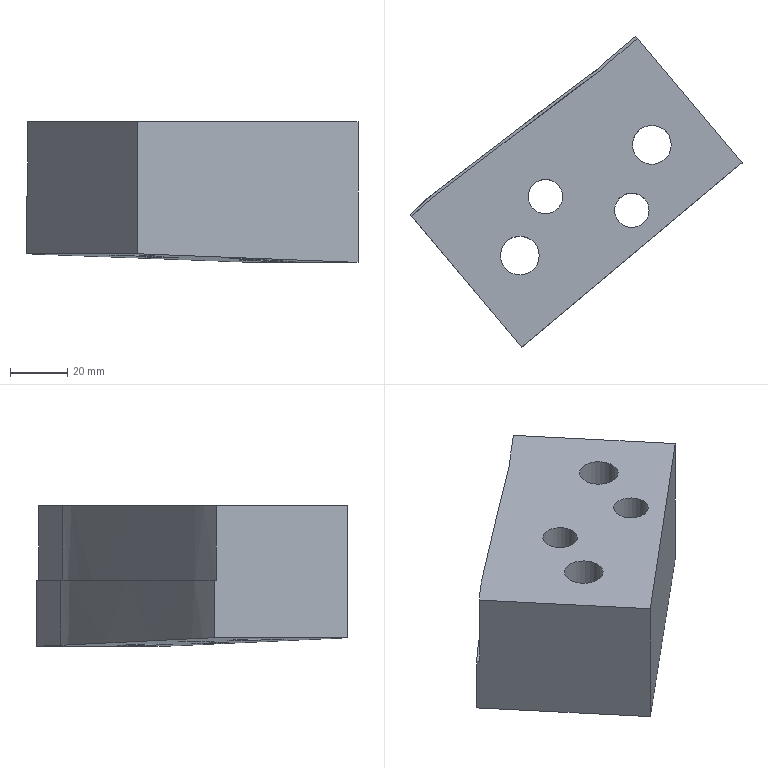Part | NX | features solid 2 | 1 solid | 22 faces | box 115.597 x 108.38 x 49 mm | volume 247805 mm3 | plane 12 | cylinder 8 | spline 2 | commonest cylinder face diameters 12 x2 13 x2 13.5 x2 19.5 x2
STEP:
#1=CARTESIAN_POINT('',(398.511,3.234,40.));
#2=VERTEX_POINT('',#1);
#3=CARTESIAN_POINT('',(408.585,11.687,40.));
#4=VERTEX_POINT('',#3);
#5=CARTESIAN_POINT('',(-63.471,-384.415,40.));
#6=DIRECTION('',(0.766,0.6428,0.));
#7=VECTOR('',#6,1000.);
#8=LINE('',#5,#7);
#9=EDGE_CURVE('',#2,#4,#8,.T.);
#10=ORIENTED_EDGE('',*,*,#9,.F.);
#11=CARTESIAN_POINT('',(329.994,-50.225,40.));
#12=VERTEX_POINT('',#11);
#13=CARTESIAN_POINT('',(329.994,-50.225,40.));
#14=CARTESIAN_POINT('',(331.334,-49.01,40.));
#15=CARTESIAN_POINT('',(333.889,-46.435,40.));
#16=CARTESIAN_POINT('',(338.043,-42.95,40.));
#17=CARTESIAN_POINT('',(342.497,-39.816,40.));
#18=CARTESIAN_POINT('',(346.834,-36.54,40.));
#19=CARTESIAN_POINT('',(351.16,-33.247,40.));
#20=CARTESIAN_POINT('',(356.896,-28.814,40.));
#21=CARTESIAN_POINT('',(364.051,-23.254,40.));
#22=CARTESIAN_POINT('',(372.649,-16.597,40.));
#23=CARTESIAN_POINT('',(379.858,-11.107,40.));
#24=CARTESIAN_POINT('',(385.676,-6.784,40.));
#25=CARTESIAN_POINT('',(390.076,-3.582,40.));
#26=CARTESIAN_POINT('',(394.468,-0.4036,40.));
#27=CARTESIAN_POINT('',(397.371,1.834,40.));
#28=CARTESIAN_POINT('',(398.511,3.234,40.));
#29=B_SPLINE_CURVE_WITH_KNOTS('',3,(#13,#14,#15,#16,#17,#18,#19,#20,#21,#22,#23,#24,#25,#26,#27,#28),.UNSPECIFIED.,.F.,.F.,(4,1,1,1,1,1,1,1,1,1,1,1,1,4),(0.001774,0.007197,0.01262,0.01804,0.02346,0.02889,0.03431,0.04515,0.056,0.06685,0.07227,0.07769,0.08311,0.08854),.UNSPECIFIED.);
#30=EDGE_CURVE('',#12,#2,#29,.T.);
#31=ORIENTED_EDGE('',*,*,#30,.F.);
#32=CARTESIAN_POINT('',(368.343,-95.927,40.));
#33=VERTEX_POINT('',#32);
#34=CARTESIAN_POINT('',(-20.026,366.913,40.));
#35=DIRECTION('',(-0.6428,0.766,0.));
#36=VECTOR('',#35,1000.);
#37=LINE('',#34,#36);
#38=EDGE_CURVE('',#33,#12,#37,.T.);
#39=ORIENTED_EDGE('',*,*,#38,.F.);
#40=CARTESIAN_POINT('',(444.947,-31.649,40.));
#41=VERTEX_POINT('',#40);
#42=CARTESIAN_POINT('',(628.198,122.117,40.));
#43=DIRECTION('',(0.766,0.6428,0.));
#44=VECTOR('',#43,1000.);
#45=LINE('',#42,#44);
#46=EDGE_CURVE('',#33,#41,#45,.T.);
#47=ORIENTED_EDGE('',*,*,#46,.T.);
#48=CARTESIAN_POINT('',(56.578,431.192,40.));
#49=DIRECTION('',(-0.6428,0.766,0.));
#50=VECTOR('',#49,1000.);
#51=LINE('',#48,#50);
#52=EDGE_CURVE('',#41,#4,#51,.T.);
#53=ORIENTED_EDGE('',*,*,#52,.T.);
#54=EDGE_LOOP('',(#10,#31,#39,#47,#53));
#55=FACE_BOUND('',#54,.T.);
#56=CARTESIAN_POINT('',(374.344,-63.92,40.));
#57=VERTEX_POINT('',#56);
#58=CARTESIAN_POINT('',(367.594,-63.92,40.));
#59=DIRECTION('',(0.,0.,1.));
#60=DIRECTION('',(1.,0.,0.));
#61=AXIS2_PLACEMENT_3D('',#58,#59,#60);
#62=CIRCLE('',#61,6.75);
#63=EDGE_CURVE('',#57,#57,#62,.T.);
#64=ORIENTED_EDGE('',*,*,#63,.F.);
#65=EDGE_LOOP('',(#64));
#66=FACE_BOUND('',#65,.T.);
#67=CARTESIAN_POINT('',(420.307,-25.353,40.));
#68=VERTEX_POINT('',#67);
#69=CARTESIAN_POINT('',(413.557,-25.353,40.));
#70=DIRECTION('',(0.,0.,1.));
#71=DIRECTION('',(1.,0.,0.));
#72=AXIS2_PLACEMENT_3D('',#69,#70,#71);
#73=CIRCLE('',#72,6.75);
#74=EDGE_CURVE('',#68,#68,#73,.T.);
#75=ORIENTED_EDGE('',*,*,#74,.F.);
#76=EDGE_LOOP('',(#75));
#77=FACE_BOUND('',#76,.T.);
#78=CARTESIAN_POINT('',(412.592,-48.168,40.));
#79=VERTEX_POINT('',#78);
#80=CARTESIAN_POINT('',(406.592,-48.168,40.));
#81=DIRECTION('',(0.,0.,1.));
#82=DIRECTION('',(1.,0.,0.));
#83=AXIS2_PLACEMENT_3D('',#80,#81,#82);
#84=CIRCLE('',#83,6.);
#85=EDGE_CURVE('',#79,#79,#84,.T.);
#86=ORIENTED_EDGE('',*,*,#85,.F.);
#87=EDGE_LOOP('',(#86));
#88=FACE_BOUND('',#87,.T.);
#89=CARTESIAN_POINT('',(382.487,-43.404,40.));
#90=VERTEX_POINT('',#89);
#91=CARTESIAN_POINT('',(376.487,-43.404,40.));
#92=DIRECTION('',(0.,0.,1.));
#93=DIRECTION('',(1.,0.,0.));
#94=AXIS2_PLACEMENT_3D('',#91,#92,#93);
#95=CIRCLE('',#94,6.);
#96=EDGE_CURVE('',#90,#90,#95,.T.);
#97=ORIENTED_EDGE('',*,*,#96,.F.);
#98=EDGE_LOOP('',(#97));
#99=FACE_BOUND('',#98,.T.);
#100=CARTESIAN_POINT('',(-415.478,35.09,40.));
#101=DIRECTION('',(0.,0.,1.));
#102=DIRECTION('',(1.,0.,0.));
#103=AXIS2_PLACEMENT_3D('',#100,#101,#102);
#104=PLANE('',#103);
#105=ADVANCED_FACE('',(#55,#66,#77,#88,#99),#104,.T.);
#106=CARTESIAN_POINT('',(397.794,3.938,14.));
#107=VERTEX_POINT('',#106);
#108=CARTESIAN_POINT('',(329.35,-49.458,14.));
#109=VERTEX_POINT('',#108);
#110=CARTESIAN_POINT('',(-190.231,-121.49,14.));
#111=CARTESIAN_POINT('',(-188.654,-121.152,14.));
#112=CARTESIAN_POINT('',(-185.47,-120.627,14.));
#113=CARTESIAN_POINT('',(-180.656,-120.141,14.));
#114=CARTESIAN_POINT('',(-175.882,-119.326,14.));
#115=CARTESIAN_POINT('',(-169.679,-117.528,14.));
#116=CARTESIAN_POINT('',(-162.185,-114.539,14.));
#117=CARTESIAN_POINT('',(-153.086,-111.254,14.));
#118=CARTESIAN_POINT('',(-144.031,-107.845,14.));
#119=CARTESIAN_POINT('',(-136.465,-105.061,14.));
#120=CARTESIAN_POINT('',(-130.418,-102.814,14.));
#121=CARTESIAN_POINT('',(-125.812,-101.329,14.));
#122=CARTESIAN_POINT('',(-121.306,-99.566,14.));
#123=CARTESIAN_POINT('',(-116.876,-97.626,14.));
#124=CARTESIAN_POINT('',(-112.335,-95.923,14.));
#125=CARTESIAN_POINT('',(-107.564,-95.05,14.));
#126=CARTESIAN_POINT('',(-102.756,-94.525,14.));
#127=CARTESIAN_POINT('',(-96.349,-93.771,14.));
#128=CARTESIAN_POINT('',(-89.902,-93.468,14.));
#129=CARTESIAN_POINT('',(-83.452,-93.448,14.));
#130=CARTESIAN_POINT('',(-77.002,-93.469,14.));
#131=CARTESIAN_POINT('',(-68.939,-93.411,14.));
#132=CARTESIAN_POINT('',(-56.04,-93.3,14.));
#133=CARTESIAN_POINT('',(-33.465,-93.184,14.));
#134=CARTESIAN_POINT('',(-7.666,-93.074,14.));
#135=CARTESIAN_POINT('',(14.907,-92.653,14.));
#136=CARTESIAN_POINT('',(27.794,-92.068,14.));
#137=CARTESIAN_POINT('',(40.668,-91.245,14.));
#138=CARTESIAN_POINT('',(51.917,-90.291,14.));
#139=CARTESIAN_POINT('',(61.528,-89.174,14.));
#140=CARTESIAN_POINT('',(67.939,-88.466,14.));
#141=CARTESIAN_POINT('',(79.125,-86.95,14.));
#142=CARTESIAN_POINT('',(95.161,-85.253,14.));
#143=CARTESIAN_POINT('',(114.404,-83.21,14.));
#144=CARTESIAN_POINT('',(133.568,-80.524,14.));
#145=CARTESIAN_POINT('',(152.734,-77.861,14.));
#146=CARTESIAN_POINT('',(171.916,-75.326,14.));
#147=CARTESIAN_POINT('',(191.055,-72.413,14.));
#148=CARTESIAN_POINT('',(207.17,-71.468,14.));
#149=CARTESIAN_POINT('',(219.951,-69.697,14.));
#150=CARTESIAN_POINT('',(232.724,-67.899,14.));
#151=CARTESIAN_POINT('',(248.708,-65.766,14.));
#152=CARTESIAN_POINT('',(267.87,-63.074,14.));
#153=CARTESIAN_POINT('',(287.038,-60.44,14.));
#154=CARTESIAN_POINT('',(301.448,-58.682,14.));
#155=CARTESIAN_POINT('',(310.976,-56.987,14.));
#156=CARTESIAN_POINT('',(314.916,-56.135,14.));
#157=CARTESIAN_POINT('',(318.052,-55.382,14.));
#158=CARTESIAN_POINT('',(320.39,-54.76,14.));
#159=CARTESIAN_POINT('',(322.686,-53.981,14.));
#160=CARTESIAN_POINT('',(325.595,-52.578,14.));
#161=CARTESIAN_POINT('',(328.769,-50.098,14.));
#162=CARTESIAN_POINT('',(332.247,-46.69,14.));
#163=CARTESIAN_POINT('',(335.795,-43.406,14.));
#164=CARTESIAN_POINT('',(343.661,-37.758,14.));
#165=CARTESIAN_POINT('',(355.164,-28.914,14.));
#166=CARTESIAN_POINT('',(370.422,-17.018,14.));
#167=CARTESIAN_POINT('',(383.264,-7.249,14.));
#168=CARTESIAN_POINT('',(392.416,-0.6713,14.));
#169=CARTESIAN_POINT('',(396.953,2.733,14.));
#170=CARTESIAN_POINT('',(398.886,5.372,14.));
#171=CARTESIAN_POINT('',(399.725,7.654,14.));
#172=CARTESIAN_POINT('',(399.76,10.078,14.));
#173=CARTESIAN_POINT('',(399.483,13.317,14.));
#174=CARTESIAN_POINT('',(399.712,17.34,14.));
#175=CARTESIAN_POINT('',(399.612,22.179,14.));
#176=CARTESIAN_POINT('',(399.633,31.854,14.));
#177=CARTESIAN_POINT('',(399.593,46.366,14.));
#178=CARTESIAN_POINT('',(399.637,62.491,14.));
#179=CARTESIAN_POINT('',(399.588,73.779,14.));
#180=CARTESIAN_POINT('',(399.652,79.422,14.));
#181=CARTESIAN_POINT('',(399.59,82.647,14.));
#182=CARTESIAN_POINT('',(399.564,85.065,14.));
#183=CARTESIAN_POINT('',(399.725,87.486,14.));
#184=CARTESIAN_POINT('',(399.756,89.902,14.));
#185=CARTESIAN_POINT('',(399.247,92.301,14.));
#186=CARTESIAN_POINT('',(397.362,95.008,14.));
#187=CARTESIAN_POINT('',(393.635,96.774,14.));
#188=CARTESIAN_POINT('',(389.279,98.826,14.));
#189=CARTESIAN_POINT('',(384.732,100.498,14.));
#190=CARTESIAN_POINT('',(378.765,102.95,14.));
#191=CARTESIAN_POINT('',(362.589,110.229,14.));
#192=CARTESIAN_POINT('',(344.928,118.135,14.));
#193=CARTESIAN_POINT('',(327.281,126.072,14.));
#194=CARTESIAN_POINT('',(319.932,129.381,14.));
#195=CARTESIAN_POINT('',(314.075,132.102,14.));
#196=CARTESIAN_POINT('',(309.387,133.376,14.));
#197=CARTESIAN_POINT('',(304.547,133.785,14.));
#198=CARTESIAN_POINT('',(299.716,133.401,14.));
#199=CARTESIAN_POINT('',(294.929,132.704,14.));
#200=CARTESIAN_POINT('',(288.543,131.8,14.));
#201=CARTESIAN_POINT('',(277.364,130.241,14.));
#202=CARTESIAN_POINT('',(242.2,125.552,14.));
#203=CARTESIAN_POINT('',(184.637,118.048,14.));
#204=CARTESIAN_POINT('',(120.701,109.541,14.));
#205=CARTESIAN_POINT('',(69.531,102.902,14.));
#206=CARTESIAN_POINT('',(40.777,98.94,14.));
#207=CARTESIAN_POINT('',(21.566,96.615,14.));
#208=CARTESIAN_POINT('',(8.743,95.212,14.));
#209=CARTESIAN_POINT('',(-7.301,93.575,14.));
#210=CARTESIAN_POINT('',(-26.625,92.505,14.));
#211=CARTESIAN_POINT('',(-45.971,92.017,14.));
#212=CARTESIAN_POINT('',(-62.09,91.675,14.));
#213=CARTESIAN_POINT('',(-74.987,91.256,14.));
#214=CARTESIAN_POINT('',(-84.664,91.165,14.));
#215=CARTESIAN_POINT('',(-94.319,91.781,14.));
#216=CARTESIAN_POINT('',(-103.929,92.966,14.));
#217=CARTESIAN_POINT('',(-113.495,94.403,14.));
#218=CARTESIAN_POINT('',(-119.856,95.492,14.));
#219=CARTESIAN_POINT('',(-122.997,96.222,14.));
#220=B_SPLINE_CURVE_WITH_KNOTS('',3,(#110,#111,#112,#113,#114,#115,#116,#117,#118,#119,#120,#121,#122,#123,#124,#125,#126,#127,#128,#129,#130,#131,#132,#133,#134,#135,#136,#137,#138,#139,#140,#141,#142,#143,#144,#145,#146,#147,#148,#149,#150,#151,#152,#153,#154,#155,#156,#157,#158,#159,#160,#161,#162,#163,#164,#165,#166,#167,#168,#169,#170,#171,#172,#173,#174,#175,#176,#177,#178,#179,#180,#181,#182,#183,#184,#185,#186,#187,#188,#189,#190,#191,#192,#193,#194,#195,#196,#197,#198,#199,#200,#201,#202,#203,#204,#205,#206,#207,#208,#209,#210,#211,#212,#213,#214,#215,#216,#217,#218,#219),.UNSPECIFIED.,.F.,.F.,(4,1,1,1,1,1,1,1,1,1,1,1,1,1,1,1,1,1,1,1,1,1,1,1,1,1,1,1,1,1,1,1,1,1,1,1,1,1,1,1,1,1,1,1,1,1,1,1,1,1,1,1,1,1,1,1,1,1,1,1,1,1,1,1,1,1,1,1,1,1,1,1,1,1,1,1,1,1,1,1,1,1,1,1,1,1,1,1,1,1,1,1,1,1,1,1,1,1,1,1,1,1,1,1,1,1,1,4),(0.4704,0.4724,0.4745,0.4766,0.4786,0.4828,0.4869,0.491,0.4952,0.4972,0.4993,0.5014,0.5035,0.5055,0.5076,0.5097,0.5117,0.5159,0.5179,0.52,0.5241,0.5283,0.5366,0.5531,0.5614,0.5655,0.5697,0.5779,0.58,0.5821,0.5862,0.5945,0.6028,0.611,0.6193,0.6276,0.6359,0.6441,0.6483,0.6524,0.6607,0.669,0.6772,0.6855,0.6876,0.6897,0.6907,0.6917,0.6928,0.6938,0.6959,0.6979,0.7,0.7021,0.7103,0.7186,0.7269,0.731,0.7331,0.7341,0.7352,0.7362,0.7372,0.7393,0.7414,0.7435,0.7517,0.76,0.7641,0.7662,0.7672,0.7683,0.7693,0.7703,0.7714,0.7724,0.7745,0.7766,0.7786,0.7807,0.7848,0.8014,0.8055,0.8097,0.8117,0.8138,0.8159,0.8179,0.82,0.8221,0.8262,0.8345,0.8676,0.9007,0.9172,0.9338,0.9379,0.9421,0.9503,0.9586,0.9669,0.9752,0.9793,0.9834,0.9876,0.9917,0.9959,1.),.UNSPECIFIED.);
#221=EDGE_CURVE('',#107,#109,#220,.F.);
#222=ORIENTED_EDGE('',*,*,#221,.F.);
#223=CARTESIAN_POINT('',(397.794,3.938,-8.603));
#224=VERTEX_POINT('',#223);
#225=CARTESIAN_POINT('',(397.794,3.938,15.353));
#226=DIRECTION('',(0.,0.,-1.));
#227=VECTOR('',#226,1000.);
#228=LINE('',#225,#227);
#229=EDGE_CURVE('',#107,#224,#228,.T.);
#230=ORIENTED_EDGE('',*,*,#229,.T.);
#231=CARTESIAN_POINT('',(329.35,-49.458,-6.));
#232=VERTEX_POINT('',#231);
#233=CARTESIAN_POINT('',(397.794,3.938,-8.603));
#234=CARTESIAN_POINT('',(396.669,2.533,-8.55));
#235=CARTESIAN_POINT('',(393.753,0.322,-8.44));
#236=CARTESIAN_POINT('',(389.372,-2.859,-8.278));
#237=CARTESIAN_POINT('',(384.978,-6.055,-8.115));
#238=CARTESIAN_POINT('',(379.17,-10.374,-7.899));
#239=CARTESIAN_POINT('',(371.973,-15.855,-7.627));
#240=CARTESIAN_POINT('',(363.39,-22.501,-7.302));
#241=CARTESIAN_POINT('',(356.247,-28.052,-7.031));
#242=CARTESIAN_POINT('',(350.521,-32.477,-6.814));
#243=CARTESIAN_POINT('',(346.202,-35.764,-6.651));
#244=CARTESIAN_POINT('',(341.87,-39.036,-6.489));
#245=CARTESIAN_POINT('',(337.427,-42.164,-6.326));
#246=CARTESIAN_POINT('',(333.263,-45.65,-6.163));
#247=CARTESIAN_POINT('',(330.694,-48.239,-6.054));
#248=CARTESIAN_POINT('',(329.35,-49.458,-6.));
#249=B_SPLINE_CURVE_WITH_KNOTS('',3,(#233,#234,#235,#236,#237,#238,#239,#240,#241,#242,#243,#244,#245,#246,#247,#248),.UNSPECIFIED.,.F.,.F.,(4,1,1,1,1,1,1,1,1,1,1,1,1,4),(0.01887,0.02429,0.02971,0.03513,0.04055,0.05139,0.06223,0.07307,0.07849,0.08391,0.08933,0.09475,0.1002,0.1056),.UNSPECIFIED.);
#250=EDGE_CURVE('',#224,#232,#249,.T.);
#251=ORIENTED_EDGE('',*,*,#250,.T.);
#252=CARTESIAN_POINT('',(329.35,-49.458,4.));
#253=DIRECTION('',(0.,0.,-1.));
#254=VECTOR('',#253,1000.);
#255=LINE('',#252,#254);
#256=EDGE_CURVE('',#109,#232,#255,.T.);
#257=ORIENTED_EDGE('',*,*,#256,.F.);
#258=EDGE_LOOP('',(#222,#230,#251,#257));
#259=FACE_BOUND('',#258,.T.);
#260=CARTESIAN_POINT('',(329.35,-49.458,14.));
#261=CARTESIAN_POINT('',(329.35,-49.458,-8.738));
#262=CARTESIAN_POINT('',(330.694,-48.239,14.));
#263=CARTESIAN_POINT('',(330.694,-48.239,-8.738));
#264=CARTESIAN_POINT('',(333.261,-45.653,14.));
#265=CARTESIAN_POINT('',(333.261,-45.653,-8.738));
#266=CARTESIAN_POINT('',(337.411,-42.175,14.));
#267=CARTESIAN_POINT('',(337.411,-42.175,-8.738));
#268=CARTESIAN_POINT('',(341.859,-39.044,14.));
#269=CARTESIAN_POINT('',(341.859,-39.044,-8.738));
#270=CARTESIAN_POINT('',(346.191,-35.773,14.));
#271=CARTESIAN_POINT('',(346.191,-35.773,-8.738));
#272=CARTESIAN_POINT('',(350.51,-32.485,14.));
#273=CARTESIAN_POINT('',(350.51,-32.485,-8.738));
#274=CARTESIAN_POINT('',(356.237,-28.06,14.));
#275=CARTESIAN_POINT('',(356.237,-28.06,-8.738));
#276=CARTESIAN_POINT('',(363.38,-22.509,14.));
#277=CARTESIAN_POINT('',(363.38,-22.509,-8.738));
#278=CARTESIAN_POINT('',(371.966,-15.861,14.));
#279=CARTESIAN_POINT('',(371.966,-15.861,-8.738));
#280=CARTESIAN_POINT('',(379.167,-10.376,14.));
#281=CARTESIAN_POINT('',(379.167,-10.376,-8.738));
#282=CARTESIAN_POINT('',(384.974,-6.058,14.));
#283=CARTESIAN_POINT('',(384.974,-6.058,-8.738));
#284=CARTESIAN_POINT('',(389.359,-2.869,14.));
#285=CARTESIAN_POINT('',(389.359,-2.869,-8.738));
#286=CARTESIAN_POINT('',(393.75,0.3223,14.));
#287=CARTESIAN_POINT('',(393.75,0.3223,-8.738));
#288=CARTESIAN_POINT('',(396.658,2.52,14.));
#289=CARTESIAN_POINT('',(396.658,2.52,-8.738));
#290=CARTESIAN_POINT('',(397.794,3.938,14.));
#291=CARTESIAN_POINT('',(397.794,3.938,-8.738));
#292=B_SPLINE_SURFACE_WITH_KNOTS('',3,1,((#260,#261),(#262,#263),(#264,#265),(#266,#267),(#268,#269),(#270,#271),(#272,#273),(#274,#275),(#276,#277),(#278,#279),(#280,#281),(#282,#283),(#284,#285),(#286,#287),(#288,#289),(#290,#291)),.SURF_OF_LINEAR_EXTRUSION.,.F.,.F.,.F.,(4,1,1,1,1,1,1,1,1,1,1,1,1,4),(2,2),(0.6962,0.6986,0.7009,0.7032,0.7055,0.7078,0.7102,0.7148,0.7194,0.7241,0.7264,0.7287,0.7311,0.7334),(0.,1.),.UNSPECIFIED.);
#293=ADVANCED_FACE('',(#259),#292,.T.);
#294=CARTESIAN_POINT('',(408.585,11.687,14.));
#295=VERTEX_POINT('',#294);
#296=CARTESIAN_POINT('',(407.942,12.453,14.));
#297=VERTEX_POINT('',#296);
#298=CARTESIAN_POINT('',(608.355,-226.39,14.));
#299=DIRECTION('',(-0.6428,0.766,0.));
#300=VECTOR('',#299,1000.);
#301=LINE('',#298,#300);
#302=EDGE_CURVE('',#295,#297,#301,.T.);
#303=ORIENTED_EDGE('',*,*,#302,.F.);
#304=CARTESIAN_POINT('',(408.585,11.687,2.));
#305=DIRECTION('',(0.,0.,-1.));
#306=VECTOR('',#305,1000.);
#307=LINE('',#304,#306);
#308=EDGE_CURVE('',#4,#295,#307,.T.);
#309=ORIENTED_EDGE('',*,*,#308,.F.);
#310=ORIENTED_EDGE('',*,*,#52,.F.);
#311=CARTESIAN_POINT('',(444.947,-31.649,-9.));
#312=VERTEX_POINT('',#311);
#313=CARTESIAN_POINT('',(444.947,-31.649,2.));
#314=DIRECTION('',(0.,0.,1.));
#315=VECTOR('',#314,1000.);
#316=LINE('',#313,#315);
#317=EDGE_CURVE('',#312,#41,#316,.T.);
#318=ORIENTED_EDGE('',*,*,#317,.F.);
#319=CARTESIAN_POINT('',(407.942,12.453,-9.));
#320=VERTEX_POINT('',#319);
#321=CARTESIAN_POINT('',(160.485,307.36,-9.));
#322=DIRECTION('',(0.6428,-0.766,0.));
#323=VECTOR('',#322,1000.);
#324=LINE('',#321,#323);
#325=EDGE_CURVE('',#320,#312,#324,.T.);
#326=ORIENTED_EDGE('',*,*,#325,.F.);
#327=CARTESIAN_POINT('',(407.942,12.453,100.));
#328=DIRECTION('',(0.,0.,1.));
#329=VECTOR('',#328,1000.);
#330=LINE('',#327,#329);
#331=EDGE_CURVE('',#297,#320,#330,.F.);
#332=ORIENTED_EDGE('',*,*,#331,.F.);
#333=EDGE_LOOP('',(#303,#309,#310,#318,#326,#332));
#334=FACE_BOUND('',#333,.T.);
#335=CARTESIAN_POINT('',(608.355,-226.39,2.));
#336=DIRECTION('',(0.766,0.6428,0.));
#337=DIRECTION('',(-0.6428,0.766,0.));
#338=AXIS2_PLACEMENT_3D('',#335,#336,#337);
#339=PLANE('',#338);
#340=ADVANCED_FACE('',(#334),#339,.T.);
#341=CARTESIAN_POINT('',(381.466,-39.226,-7.395));
#342=VERTEX_POINT('',#341);
#343=CARTESIAN_POINT('',(376.487,-43.404,-7.2));
#344=DIRECTION('',(-0.02297,-0.01927,-0.9996));
#345=DIRECTION('',(0.7657,0.6425,-0.02999));
#346=AXIS2_PLACEMENT_3D('',#343,#344,#345);
#347=ELLIPSE('',#346,6.503,6.5);
#348=EDGE_CURVE('',#342,#342,#347,.T.);
#349=ORIENTED_EDGE('',*,*,#348,.F.);
#350=EDGE_LOOP('',(#349));
#351=FACE_BOUND('',#350,.T.);
#352=CARTESIAN_POINT('',(411.571,-43.989,-7.995));
#353=VERTEX_POINT('',#352);
#354=CARTESIAN_POINT('',(406.592,-48.168,-7.8));
#355=DIRECTION('',(-0.02297,-0.01927,-0.9996));
#356=DIRECTION('',(0.7657,0.6425,-0.02999));
#357=AXIS2_PLACEMENT_3D('',#354,#355,#356);
#358=ELLIPSE('',#357,6.503,6.5);
#359=EDGE_CURVE('',#353,#353,#358,.T.);
#360=ORIENTED_EDGE('',*,*,#359,.F.);
#361=EDGE_LOOP('',(#360));
#362=FACE_BOUND('',#361,.T.);
#363=CARTESIAN_POINT('',(421.026,-19.086,-8.693));
#364=VERTEX_POINT('',#363);
#365=CARTESIAN_POINT('',(413.557,-25.353,-8.4));
#366=DIRECTION('',(-0.02297,-0.01927,-0.9996));
#367=DIRECTION('',(0.7657,0.6425,-0.02999));
#368=AXIS2_PLACEMENT_3D('',#365,#366,#367);
#369=ELLIPSE('',#368,9.754,9.75);
#370=EDGE_CURVE('',#364,#364,#369,.T.);
#371=ORIENTED_EDGE('',*,*,#370,.F.);
#372=EDGE_LOOP('',(#371));
#373=FACE_BOUND('',#372,.T.);
#374=CARTESIAN_POINT('',(375.063,-57.653,-6.893));
#375=VERTEX_POINT('',#374);
#376=CARTESIAN_POINT('',(367.594,-63.92,-6.6));
#377=DIRECTION('',(-0.02297,-0.01927,-0.9996));
#378=DIRECTION('',(0.7657,0.6425,-0.02999));
#379=AXIS2_PLACEMENT_3D('',#376,#377,#378);
#380=ELLIPSE('',#379,9.754,9.75);
#381=EDGE_CURVE('',#375,#375,#380,.T.);
#382=ORIENTED_EDGE('',*,*,#381,.F.);
#383=EDGE_LOOP('',(#382));
#384=FACE_BOUND('',#383,.T.);
#385=ORIENTED_EDGE('',*,*,#250,.F.);
#386=CARTESIAN_POINT('',(331.337,-51.826,-6.));
#387=DIRECTION('',(0.7657,0.6425,-0.02999));
#388=VECTOR('',#387,1000.);
#389=LINE('',#386,#388);
#390=EDGE_CURVE('',#224,#320,#389,.T.);
#391=ORIENTED_EDGE('',*,*,#390,.T.);
#392=ORIENTED_EDGE('',*,*,#325,.T.);
#393=CARTESIAN_POINT('',(368.343,-95.927,-6.));
#394=VERTEX_POINT('',#393);
#395=CARTESIAN_POINT('',(627.965,121.921,-16.167));
#396=DIRECTION('',(0.7657,0.6425,-0.02999));
#397=VECTOR('',#396,1000.);
#398=LINE('',#395,#397);
#399=EDGE_CURVE('',#394,#312,#398,.T.);
#400=ORIENTED_EDGE('',*,*,#399,.F.);
#401=CARTESIAN_POINT('',(83.881,243.081,-6.));
#402=DIRECTION('',(0.6428,-0.766,0.));
#403=VECTOR('',#402,1000.);
#404=LINE('',#401,#403);
#405=EDGE_CURVE('',#232,#394,#404,.T.);
#406=ORIENTED_EDGE('',*,*,#405,.F.);
#407=EDGE_LOOP('',(#385,#391,#392,#400,#406));
#408=FACE_BOUND('',#407,.T.);
#409=CARTESIAN_POINT('',(368.343,-95.927,-6.));
#410=DIRECTION('',(-0.02297,-0.01927,-0.9996));
#411=DIRECTION('',(-0.9997,0.,0.02298));
#412=AXIS2_PLACEMENT_3D('',#409,#410,#411);
#413=PLANE('',#412);
#414=ADVANCED_FACE('',(#351,#362,#373,#384,#408),#413,.T.);
#415=CARTESIAN_POINT('',(329.994,-50.225,14.));
#416=VERTEX_POINT('',#415);
#417=CARTESIAN_POINT('',(329.994,-50.225,57.));
#418=DIRECTION('',(0.,0.,1.));
#419=VECTOR('',#418,1000.);
#420=LINE('',#417,#419);
#421=EDGE_CURVE('',#12,#416,#420,.F.);
#422=ORIENTED_EDGE('',*,*,#421,.T.);
#423=CARTESIAN_POINT('',(354.158,-79.022,14.));
#424=DIRECTION('',(-0.6428,0.766,0.));
#425=VECTOR('',#424,1000.);
#426=LINE('',#423,#425);
#427=EDGE_CURVE('',#416,#109,#426,.T.);
#428=ORIENTED_EDGE('',*,*,#427,.T.);
#429=ORIENTED_EDGE('',*,*,#256,.T.);
#430=ORIENTED_EDGE('',*,*,#405,.T.);
#431=CARTESIAN_POINT('',(368.343,-95.927,23.));
#432=DIRECTION('',(0.,0.,1.));
#433=VECTOR('',#432,1000.);
#434=LINE('',#431,#433);
#435=EDGE_CURVE('',#394,#33,#434,.T.);
#436=ORIENTED_EDGE('',*,*,#435,.T.);
#437=ORIENTED_EDGE('',*,*,#38,.T.);
#438=EDGE_LOOP('',(#422,#428,#429,#430,#436,#437));
#439=FACE_BOUND('',#438,.T.);
#440=CARTESIAN_POINT('',(354.158,-79.022,23.));
#441=DIRECTION('',(0.766,0.6428,0.));
#442=DIRECTION('',(-0.6428,0.766,0.));
#443=AXIS2_PLACEMENT_3D('',#440,#441,#442);
#444=PLANE('',#443);
#445=ADVANCED_FACE('',(#439),#444,.F.);
#446=ORIENTED_EDGE('',*,*,#435,.F.);
#447=ORIENTED_EDGE('',*,*,#399,.T.);
#448=ORIENTED_EDGE('',*,*,#317,.T.);
#449=ORIENTED_EDGE('',*,*,#46,.F.);
#450=EDGE_LOOP('',(#446,#447,#448,#449));
#451=FACE_BOUND('',#450,.T.);
#452=CARTESIAN_POINT('',(628.198,122.117,2.));
#453=DIRECTION('',(-0.6428,0.766,0.));
#454=DIRECTION('',(-0.766,-0.6428,0.));
#455=AXIS2_PLACEMENT_3D('',#452,#453,#454);
#456=PLANE('',#455);
#457=ADVANCED_FACE('',(#451),#456,.F.);
#458=ORIENTED_EDGE('',*,*,#63,.T.);
#459=EDGE_LOOP('',(#458));
#460=FACE_BOUND('',#459,.T.);
#461=CARTESIAN_POINT('',(374.344,-63.92,9.));
#462=VERTEX_POINT('',#461);
#463=CARTESIAN_POINT('',(367.594,-63.92,9.));
#464=DIRECTION('',(0.,0.,1.));
#465=DIRECTION('',(1.,0.,0.));
#466=AXIS2_PLACEMENT_3D('',#463,#464,#465);
#467=CIRCLE('',#466,6.75);
#468=EDGE_CURVE('',#462,#462,#467,.T.);
#469=ORIENTED_EDGE('',*,*,#468,.F.);
#470=EDGE_LOOP('',(#469));
#471=FACE_BOUND('',#470,.T.);
#472=CARTESIAN_POINT('',(367.594,-63.92,94.));
#473=DIRECTION('',(0.,0.,1.));
#474=DIRECTION('',(1.,0.,0.));
#475=AXIS2_PLACEMENT_3D('',#472,#473,#474);
#476=CYLINDRICAL_SURFACE('',#475,6.75);
#477=ADVANCED_FACE('',(#460,#471),#476,.F.);
#478=ORIENTED_EDGE('',*,*,#468,.T.);
#479=EDGE_LOOP('',(#478));
#480=FACE_BOUND('',#479,.T.);
#481=CARTESIAN_POINT('',(377.344,-63.92,9.));
#482=VERTEX_POINT('',#481);
#483=CARTESIAN_POINT('',(367.594,-63.92,9.));
#484=DIRECTION('',(0.,0.,1.));
#485=DIRECTION('',(1.,0.,0.));
#486=AXIS2_PLACEMENT_3D('',#483,#484,#485);
#487=CIRCLE('',#486,9.75);
#488=EDGE_CURVE('',#482,#482,#487,.T.);
#489=ORIENTED_EDGE('',*,*,#488,.F.);
#490=EDGE_LOOP('',(#489));
#491=FACE_BOUND('',#490,.T.);
#492=CARTESIAN_POINT('',(367.594,-63.92,9.));
#493=DIRECTION('',(0.,0.,1.));
#494=DIRECTION('',(1.,0.,0.));
#495=AXIS2_PLACEMENT_3D('',#492,#493,#494);
#496=PLANE('',#495);
#497=ADVANCED_FACE('',(#480,#491),#496,.F.);
#498=ORIENTED_EDGE('',*,*,#488,.T.);
#499=EDGE_LOOP('',(#498));
#500=FACE_BOUND('',#499,.T.);
#501=ORIENTED_EDGE('',*,*,#381,.T.);
#502=EDGE_LOOP('',(#501));
#503=FACE_BOUND('',#502,.T.);
#504=CARTESIAN_POINT('',(367.594,-63.92,-6.));
#505=DIRECTION('',(0.,0.,1.));
#506=DIRECTION('',(1.,0.,0.));
#507=AXIS2_PLACEMENT_3D('',#504,#505,#506);
#508=CYLINDRICAL_SURFACE('',#507,9.75);
#509=ADVANCED_FACE('',(#500,#503),#508,.F.);
#510=ORIENTED_EDGE('',*,*,#74,.T.);
#511=EDGE_LOOP('',(#510));
#512=FACE_BOUND('',#511,.T.);
#513=CARTESIAN_POINT('',(420.307,-25.353,9.));
#514=VERTEX_POINT('',#513);
#515=CARTESIAN_POINT('',(413.557,-25.353,9.));
#516=DIRECTION('',(0.,0.,1.));
#517=DIRECTION('',(1.,0.,0.));
#518=AXIS2_PLACEMENT_3D('',#515,#516,#517);
#519=CIRCLE('',#518,6.75);
#520=EDGE_CURVE('',#514,#514,#519,.T.);
#521=ORIENTED_EDGE('',*,*,#520,.F.);
#522=EDGE_LOOP('',(#521));
#523=FACE_BOUND('',#522,.T.);
#524=CARTESIAN_POINT('',(413.557,-25.353,94.));
#525=DIRECTION('',(0.,0.,1.));
#526=DIRECTION('',(1.,0.,0.));
#527=AXIS2_PLACEMENT_3D('',#524,#525,#526);
#528=CYLINDRICAL_SURFACE('',#527,6.75);
#529=ADVANCED_FACE('',(#512,#523),#528,.F.);
#530=ORIENTED_EDGE('',*,*,#520,.T.);
#531=EDGE_LOOP('',(#530));
#532=FACE_BOUND('',#531,.T.);
#533=CARTESIAN_POINT('',(423.307,-25.353,9.));
#534=VERTEX_POINT('',#533);
#535=CARTESIAN_POINT('',(413.557,-25.353,9.));
#536=DIRECTION('',(0.,0.,1.));
#537=DIRECTION('',(1.,0.,0.));
#538=AXIS2_PLACEMENT_3D('',#535,#536,#537);
#539=CIRCLE('',#538,9.75);
#540=EDGE_CURVE('',#534,#534,#539,.T.);
#541=ORIENTED_EDGE('',*,*,#540,.F.);
#542=EDGE_LOOP('',(#541));
#543=FACE_BOUND('',#542,.T.);
#544=CARTESIAN_POINT('',(413.557,-25.353,9.));
#545=DIRECTION('',(0.,0.,1.));
#546=DIRECTION('',(1.,0.,0.));
#547=AXIS2_PLACEMENT_3D('',#544,#545,#546);
#548=PLANE('',#547);
#549=ADVANCED_FACE('',(#532,#543),#548,.F.);
#550=ORIENTED_EDGE('',*,*,#540,.T.);
#551=EDGE_LOOP('',(#550));
#552=FACE_BOUND('',#551,.T.);
#553=ORIENTED_EDGE('',*,*,#370,.T.);
#554=EDGE_LOOP('',(#553));
#555=FACE_BOUND('',#554,.T.);
#556=CARTESIAN_POINT('',(413.557,-25.353,-6.));
#557=DIRECTION('',(0.,0.,1.));
#558=DIRECTION('',(1.,0.,0.));
#559=AXIS2_PLACEMENT_3D('',#556,#557,#558);
#560=CYLINDRICAL_SURFACE('',#559,9.75);
#561=ADVANCED_FACE('',(#552,#555),#560,.F.);
#562=ORIENTED_EDGE('',*,*,#85,.T.);
#563=EDGE_LOOP('',(#562));
#564=FACE_BOUND('',#563,.T.);
#565=CARTESIAN_POINT('',(412.592,-48.168,14.));
#566=VERTEX_POINT('',#565);
#567=CARTESIAN_POINT('',(406.592,-48.168,14.));
#568=DIRECTION('',(0.,0.,1.));
#569=DIRECTION('',(1.,0.,0.));
#570=AXIS2_PLACEMENT_3D('',#567,#568,#569);
#571=CIRCLE('',#570,6.);
#572=EDGE_CURVE('',#566,#566,#571,.T.);
#573=ORIENTED_EDGE('',*,*,#572,.F.);
#574=EDGE_LOOP('',(#573));
#575=FACE_BOUND('',#574,.T.);
#576=CARTESIAN_POINT('',(406.592,-48.168,94.));
#577=DIRECTION('',(0.,0.,1.));
#578=DIRECTION('',(1.,0.,0.));
#579=AXIS2_PLACEMENT_3D('',#576,#577,#578);
#580=CYLINDRICAL_SURFACE('',#579,6.);
#581=ADVANCED_FACE('',(#564,#575),#580,.F.);
#582=ORIENTED_EDGE('',*,*,#572,.T.);
#583=EDGE_LOOP('',(#582));
#584=FACE_BOUND('',#583,.T.);
#585=CARTESIAN_POINT('',(413.092,-48.168,14.));
#586=VERTEX_POINT('',#585);
#587=CARTESIAN_POINT('',(406.592,-48.168,14.));
#588=DIRECTION('',(0.,0.,1.));
#589=DIRECTION('',(1.,0.,0.));
#590=AXIS2_PLACEMENT_3D('',#587,#588,#589);
#591=CIRCLE('',#590,6.5);
#592=EDGE_CURVE('',#586,#586,#591,.T.);
#593=ORIENTED_EDGE('',*,*,#592,.F.);
#594=EDGE_LOOP('',(#593));
#595=FACE_BOUND('',#594,.T.);
#596=CARTESIAN_POINT('',(406.592,-48.168,14.));
#597=DIRECTION('',(0.,0.,1.));
#598=DIRECTION('',(1.,0.,0.));
#599=AXIS2_PLACEMENT_3D('',#596,#597,#598);
#600=PLANE('',#599);
#601=ADVANCED_FACE('',(#584,#595),#600,.F.);
#602=ORIENTED_EDGE('',*,*,#592,.T.);
#603=EDGE_LOOP('',(#602));
#604=FACE_BOUND('',#603,.T.);
#605=ORIENTED_EDGE('',*,*,#359,.T.);
#606=EDGE_LOOP('',(#605));
#607=FACE_BOUND('',#606,.T.);
#608=CARTESIAN_POINT('',(406.592,-48.168,-6.));
#609=DIRECTION('',(0.,0.,1.));
#610=DIRECTION('',(1.,0.,0.));
#611=AXIS2_PLACEMENT_3D('',#608,#609,#610);
#612=CYLINDRICAL_SURFACE('',#611,6.5);
#613=ADVANCED_FACE('',(#604,#607),#612,.F.);
#614=ORIENTED_EDGE('',*,*,#96,.T.);
#615=EDGE_LOOP('',(#614));
#616=FACE_BOUND('',#615,.T.);
#617=CARTESIAN_POINT('',(382.487,-43.404,14.));
#618=VERTEX_POINT('',#617);
#619=CARTESIAN_POINT('',(376.487,-43.404,14.));
#620=DIRECTION('',(0.,0.,1.));
#621=DIRECTION('',(1.,0.,0.));
#622=AXIS2_PLACEMENT_3D('',#619,#620,#621);
#623=CIRCLE('',#622,6.);
#624=EDGE_CURVE('',#618,#618,#623,.T.);
#625=ORIENTED_EDGE('',*,*,#624,.F.);
#626=EDGE_LOOP('',(#625));
#627=FACE_BOUND('',#626,.T.);
#628=CARTESIAN_POINT('',(376.487,-43.404,94.));
#629=DIRECTION('',(0.,0.,1.));
#630=DIRECTION('',(1.,0.,0.));
#631=AXIS2_PLACEMENT_3D('',#628,#629,#630);
#632=CYLINDRICAL_SURFACE('',#631,6.);
#633=ADVANCED_FACE('',(#616,#627),#632,.F.);
#634=ORIENTED_EDGE('',*,*,#624,.T.);
#635=EDGE_LOOP('',(#634));
#636=FACE_BOUND('',#635,.T.);
#637=CARTESIAN_POINT('',(382.987,-43.404,14.));
#638=VERTEX_POINT('',#637);
#639=CARTESIAN_POINT('',(376.487,-43.404,14.));
#640=DIRECTION('',(0.,0.,1.));
#641=DIRECTION('',(1.,0.,0.));
#642=AXIS2_PLACEMENT_3D('',#639,#640,#641);
#643=CIRCLE('',#642,6.5);
#644=EDGE_CURVE('',#638,#638,#643,.T.);
#645=ORIENTED_EDGE('',*,*,#644,.F.);
#646=EDGE_LOOP('',(#645));
#647=FACE_BOUND('',#646,.T.);
#648=CARTESIAN_POINT('',(376.487,-43.404,14.));
#649=DIRECTION('',(0.,0.,1.));
#650=DIRECTION('',(1.,0.,0.));
#651=AXIS2_PLACEMENT_3D('',#648,#649,#650);
#652=PLANE('',#651);
#653=ADVANCED_FACE('',(#636,#647),#652,.F.);
#654=ORIENTED_EDGE('',*,*,#644,.T.);
#655=EDGE_LOOP('',(#654));
#656=FACE_BOUND('',#655,.T.);
#657=ORIENTED_EDGE('',*,*,#348,.T.);
#658=EDGE_LOOP('',(#657));
#659=FACE_BOUND('',#658,.T.);
#660=CARTESIAN_POINT('',(376.487,-43.404,-6.));
#661=DIRECTION('',(0.,0.,1.));
#662=DIRECTION('',(1.,0.,0.));
#663=AXIS2_PLACEMENT_3D('',#660,#661,#662);
#664=CYLINDRICAL_SURFACE('',#663,6.5);
#665=ADVANCED_FACE('',(#656,#659),#664,.F.);
#666=CARTESIAN_POINT('',(386.216,-5.777,14.));
#667=DIRECTION('',(-0.766,-0.6428,0.));
#668=VECTOR('',#667,1000.);
#669=LINE('',#666,#668);
#670=EDGE_CURVE('',#297,#107,#669,.T.);
#671=ORIENTED_EDGE('',*,*,#670,.F.);
#672=ORIENTED_EDGE('',*,*,#331,.T.);
#673=ORIENTED_EDGE('',*,*,#390,.F.);
#674=ORIENTED_EDGE('',*,*,#229,.F.);
#675=EDGE_LOOP('',(#671,#672,#673,#674));
#676=FACE_BOUND('',#675,.T.);
#677=CARTESIAN_POINT('',(386.216,-5.777,100.));
#678=DIRECTION('',(-0.6428,0.766,0.));
#679=DIRECTION('',(-0.766,-0.6428,0.));
#680=AXIS2_PLACEMENT_3D('',#677,#678,#679);
#681=PLANE('',#680);
#682=ADVANCED_FACE('',(#676),#681,.T.);
#683=ORIENTED_EDGE('',*,*,#221,.T.);
#684=ORIENTED_EDGE('',*,*,#427,.F.);
#685=CARTESIAN_POINT('',(398.511,3.234,14.));
#686=VERTEX_POINT('',#685);
#687=CARTESIAN_POINT('',(329.994,-50.225,14.));
#688=CARTESIAN_POINT('',(331.361,-48.985,14.));
#689=CARTESIAN_POINT('',(333.935,-46.396,14.));
#690=CARTESIAN_POINT('',(337.952,-43.02,14.));
#691=CARTESIAN_POINT('',(342.416,-39.875,14.));
#692=CARTESIAN_POINT('',(346.752,-36.602,14.));
#693=CARTESIAN_POINT('',(351.076,-33.311,14.));
#694=CARTESIAN_POINT('',(356.803,-28.886,14.));
#695=CARTESIAN_POINT('',(363.943,-23.339,14.));
#696=CARTESIAN_POINT('',(372.519,-16.697,14.));
#697=CARTESIAN_POINT('',(379.709,-11.22,14.));
#698=CARTESIAN_POINT('',(385.498,-6.914,14.));
#699=CARTESIAN_POINT('',(389.885,-3.725,14.));
#700=CARTESIAN_POINT('',(394.236,-0.5524,14.));
#701=CARTESIAN_POINT('',(397.264,1.703,14.));
#702=CARTESIAN_POINT('',(398.511,3.234,14.));
#703=B_SPLINE_CURVE_WITH_KNOTS('',3,(#687,#688,#689,#690,#691,#692,#693,#694,#695,#696,#697,#698,#699,#700,#701,#702),.UNSPECIFIED.,.F.,.F.,(4,1,1,1,1,1,1,1,1,1,1,1,1,4),(0.6962,0.6985,0.7009,0.7032,0.7055,0.7078,0.7101,0.7148,0.7194,0.7241,0.7264,0.7287,0.731,0.7333),.UNSPECIFIED.);
#704=EDGE_CURVE('',#416,#686,#703,.T.);
#705=ORIENTED_EDGE('',*,*,#704,.T.);
#706=CARTESIAN_POINT('',(398.437,3.172,14.));
#707=DIRECTION('',(0.766,0.6428,0.));
#708=VECTOR('',#707,1000.);
#709=LINE('',#706,#708);
#710=EDGE_CURVE('',#686,#295,#709,.T.);
#711=ORIENTED_EDGE('',*,*,#710,.T.);
#712=ORIENTED_EDGE('',*,*,#302,.T.);
#713=ORIENTED_EDGE('',*,*,#670,.T.);
#714=EDGE_LOOP('',(#683,#684,#705,#711,#712,#713));
#715=FACE_BOUND('',#714,.T.);
#716=CARTESIAN_POINT('',(-190.231,-121.49,14.));
#717=DIRECTION('',(0.,0.,-1.));
#718=DIRECTION('',(-1.,0.,0.));
#719=AXIS2_PLACEMENT_3D('',#716,#717,#718);
#720=PLANE('',#719);
#721=ADVANCED_FACE('',(#715),#720,.F.);
#722=ORIENTED_EDGE('',*,*,#30,.T.);
#723=CARTESIAN_POINT('',(398.511,3.234,27.));
#724=DIRECTION('',(0.,0.,1.));
#725=VECTOR('',#724,1000.);
#726=LINE('',#723,#725);
#727=EDGE_CURVE('',#2,#686,#726,.F.);
#728=ORIENTED_EDGE('',*,*,#727,.T.);
#729=ORIENTED_EDGE('',*,*,#704,.F.);
#730=ORIENTED_EDGE('',*,*,#421,.F.);
#731=EDGE_LOOP('',(#722,#728,#729,#730));
#732=FACE_BOUND('',#731,.T.);
#733=CARTESIAN_POINT('',(329.994,-50.225,14.));
#734=CARTESIAN_POINT('',(329.994,-50.225,40.));
#735=CARTESIAN_POINT('',(331.361,-48.985,14.));
#736=CARTESIAN_POINT('',(331.361,-48.985,40.));
#737=CARTESIAN_POINT('',(333.935,-46.396,14.));
#738=CARTESIAN_POINT('',(333.935,-46.396,40.));
#739=CARTESIAN_POINT('',(337.952,-43.02,14.));
#740=CARTESIAN_POINT('',(337.952,-43.02,40.));
#741=CARTESIAN_POINT('',(342.416,-39.875,14.));
#742=CARTESIAN_POINT('',(342.416,-39.875,40.));
#743=CARTESIAN_POINT('',(346.752,-36.602,14.));
#744=CARTESIAN_POINT('',(346.752,-36.602,40.));
#745=CARTESIAN_POINT('',(351.076,-33.311,14.));
#746=CARTESIAN_POINT('',(351.076,-33.311,40.));
#747=CARTESIAN_POINT('',(356.803,-28.886,14.));
#748=CARTESIAN_POINT('',(356.803,-28.886,40.));
#749=CARTESIAN_POINT('',(363.943,-23.339,14.));
#750=CARTESIAN_POINT('',(363.943,-23.339,40.));
#751=CARTESIAN_POINT('',(372.519,-16.697,14.));
#752=CARTESIAN_POINT('',(372.519,-16.697,40.));
#753=CARTESIAN_POINT('',(379.709,-11.22,14.));
#754=CARTESIAN_POINT('',(379.709,-11.22,40.));
#755=CARTESIAN_POINT('',(385.498,-6.914,14.));
#756=CARTESIAN_POINT('',(385.498,-6.914,40.));
#757=CARTESIAN_POINT('',(389.885,-3.725,14.));
#758=CARTESIAN_POINT('',(389.885,-3.725,40.));
#759=CARTESIAN_POINT('',(394.236,-0.5524,14.));
#760=CARTESIAN_POINT('',(394.236,-0.5524,40.));
#761=CARTESIAN_POINT('',(397.264,1.703,14.));
#762=CARTESIAN_POINT('',(397.264,1.703,40.));
#763=CARTESIAN_POINT('',(398.511,3.234,14.));
#764=CARTESIAN_POINT('',(398.511,3.234,40.));
#765=B_SPLINE_SURFACE_WITH_KNOTS('',3,1,((#733,#734),(#735,#736),(#737,#738),(#739,#740),(#741,#742),(#743,#744),(#745,#746),(#747,#748),(#749,#750),(#751,#752),(#753,#754),(#755,#756),(#757,#758),(#759,#760),(#761,#762),(#763,#764)),.SURF_OF_LINEAR_EXTRUSION.,.F.,.F.,.F.,(4,1,1,1,1,1,1,1,1,1,1,1,1,4),(2,2),(0.6962,0.6985,0.7009,0.7032,0.7055,0.7078,0.7101,0.7148,0.7194,0.7241,0.7264,0.7287,0.731,0.7333),(0.,1.),.UNSPECIFIED.);
#766=ADVANCED_FACE('',(#732),#765,.F.);
#767=ORIENTED_EDGE('',*,*,#308,.T.);
#768=ORIENTED_EDGE('',*,*,#710,.F.);
#769=ORIENTED_EDGE('',*,*,#727,.F.);
#770=ORIENTED_EDGE('',*,*,#9,.T.);
#771=EDGE_LOOP('',(#767,#768,#769,#770));
#772=FACE_BOUND('',#771,.T.);
#773=CARTESIAN_POINT('',(398.437,3.172,13.397));
#774=DIRECTION('',(0.6428,-0.766,0.));
#775=DIRECTION('',(0.766,0.6428,0.));
#776=AXIS2_PLACEMENT_3D('',#773,#774,#775);
#777=PLANE('',#776);
#778=ADVANCED_FACE('',(#772),#777,.F.);
#779=CLOSED_SHELL('',(#105,#293,#340,#414,#445,#457,#477,#497,#509,#529,#549,#561,#581,#601,#613,#633,#653,#665,#682,#721,#766,#778));
#780=MANIFOLD_SOLID_BREP('',#779);
#781=(LENGTH_UNIT()NAMED_UNIT(*)SI_UNIT(.MILLI.,.METRE.));
#782=UNCERTAINTY_MEASURE_WITH_UNIT(LENGTH_MEASURE(0.0508),#781,'','');
#783=(NAMED_UNIT(*)PLANE_ANGLE_UNIT()SI_UNIT($,.RADIAN.));
#784=(NAMED_UNIT(*)SI_UNIT($,.STERADIAN.)SOLID_ANGLE_UNIT());
#785=(GEOMETRIC_REPRESENTATION_CONTEXT(3)GLOBAL_UNCERTAINTY_ASSIGNED_CONTEXT((#782))GLOBAL_UNIT_ASSIGNED_CONTEXT((#781,#783,#784))REPRESENTATION_CONTEXT('',''));
#786=ADVANCED_BREP_SHAPE_REPRESENTATION('',(#780),#785);